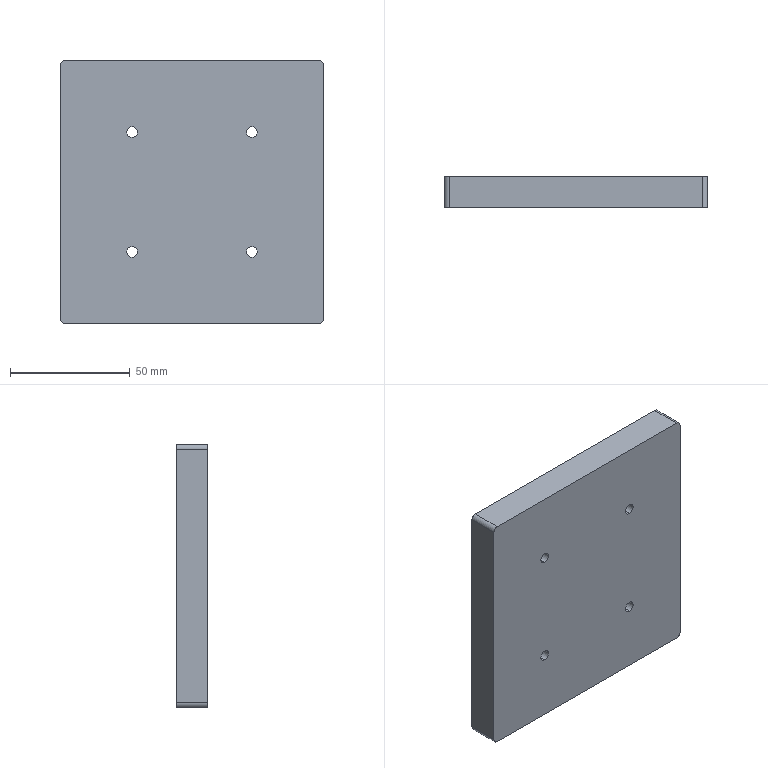Part | STEP file | Ejector Urethane Pad_Default | 1 solid | 30 faces | box 110 x 13 x 110 mm | volume 155824 mm3 | cylinder 20 | plane 10 | commonest cylinder face diameters 4.5 x8 8 x8 4 x4